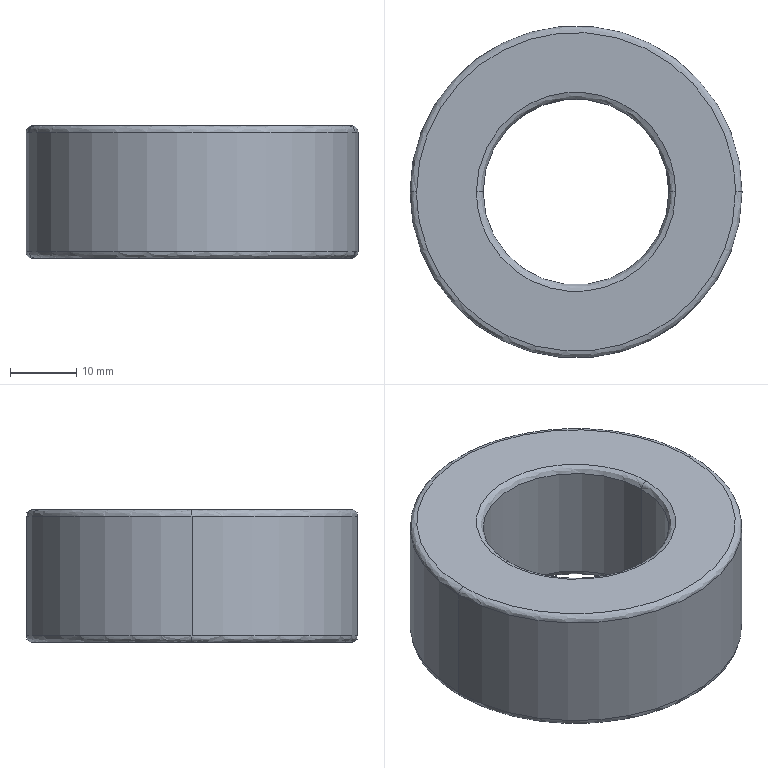Part | STEP file | Buffer sleeve | 1 solid | 14 faces | box 50 x 50 x 20 mm | volume 26853 mm3 | spline 8 | cylinder 4 | plane 2 | commonest cylinder face diameters 28 x2 50 x2